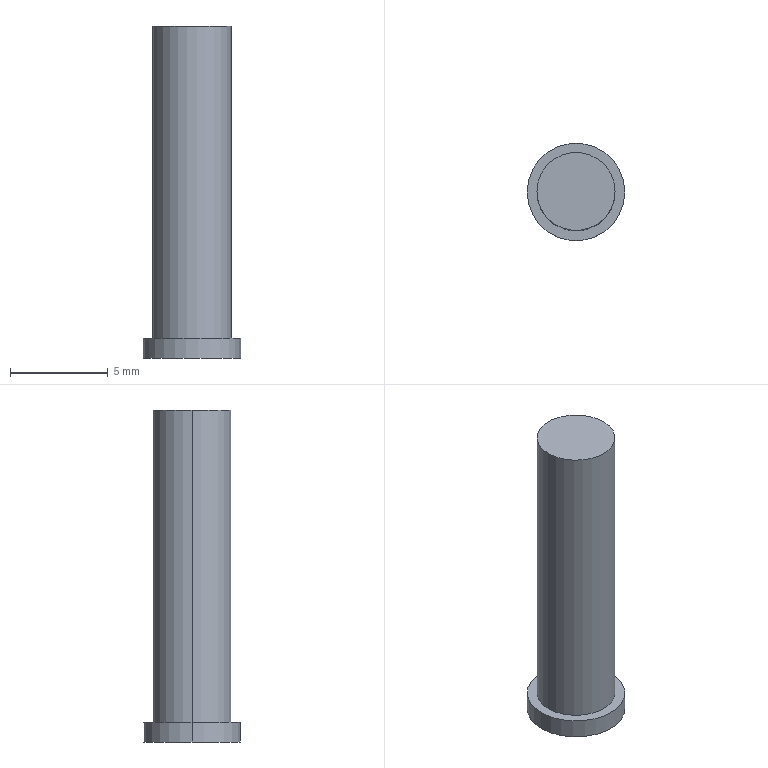Part | SolidWorks | features Extrusion 1, ICE 1 | 1 solid | 7 faces | box 5 x 5 x 17 mm | volume 220.697 mm3 | cylinder 4 | plane 3 | commonest cylinder face diameters 4 x2 5 x2
STEP:
#1=CARTESIAN_POINT('',(2.,0.,17.));
#2=VERTEX_POINT('',#1);
#3=CARTESIAN_POINT('',(-2.,0.,17.));
#4=VERTEX_POINT('',#3);
#5=CARTESIAN_POINT('',(0.,0.,17.));
#6=DIRECTION('',(0.,0.,1.));
#7=DIRECTION('',(1.,0.,0.));
#8=AXIS2_PLACEMENT_3D('',#5,#6,#7);
#9=CIRCLE('',#8,2.);
#10=EDGE_CURVE('',#2,#4,#9,.T.);
#11=ORIENTED_EDGE('',*,*,#10,.F.);
#12=CARTESIAN_POINT('',(2.,0.,1.));
#13=VERTEX_POINT('',#12);
#14=CARTESIAN_POINT('',(2.,0.,17.));
#15=DIRECTION('',(0.,0.,-1.));
#16=VECTOR('',#15,1000.);
#17=LINE('',#14,#16);
#18=EDGE_CURVE('',#2,#13,#17,.T.);
#19=ORIENTED_EDGE('',*,*,#18,.T.);
#20=CARTESIAN_POINT('',(-2.,0.,1.));
#21=VERTEX_POINT('',#20);
#22=CARTESIAN_POINT('',(0.,0.,1.));
#23=DIRECTION('',(0.,0.,1.));
#24=DIRECTION('',(1.,0.,0.));
#25=AXIS2_PLACEMENT_3D('',#22,#23,#24);
#26=CIRCLE('',#25,2.);
#27=EDGE_CURVE('',#13,#21,#26,.T.);
#28=ORIENTED_EDGE('',*,*,#27,.T.);
#29=CARTESIAN_POINT('',(-2.,0.,17.));
#30=DIRECTION('',(0.,0.,-1.));
#31=VECTOR('',#30,1000.);
#32=LINE('',#29,#31);
#33=EDGE_CURVE('',#4,#21,#32,.T.);
#34=ORIENTED_EDGE('',*,*,#33,.F.);
#35=EDGE_LOOP('',(#11,#19,#28,#34));
#36=FACE_OUTER_BOUND('',#35,.T.);
#37=CARTESIAN_POINT('',(0.,0.,17.));
#38=DIRECTION('',(0.,0.,-1.));
#39=DIRECTION('',(-1.,0.,0.));
#40=AXIS2_PLACEMENT_3D('',#37,#38,#39);
#41=CYLINDRICAL_SURFACE('',#40,2.);
#42=ADVANCED_FACE('',(#36),#41,.T.);
#43=CARTESIAN_POINT('',(2.5,0.,1.));
#44=VERTEX_POINT('',#43);
#45=CARTESIAN_POINT('',(-2.5,0.,1.));
#46=VERTEX_POINT('',#45);
#47=CARTESIAN_POINT('',(0.,0.,1.));
#48=DIRECTION('',(0.,0.,1.));
#49=DIRECTION('',(1.,0.,0.));
#50=AXIS2_PLACEMENT_3D('',#47,#48,#49);
#51=CIRCLE('',#50,2.5);
#52=EDGE_CURVE('',#44,#46,#51,.T.);
#53=ORIENTED_EDGE('',*,*,#52,.F.);
#54=CARTESIAN_POINT('',(2.5,0.,0.));
#55=VERTEX_POINT('',#54);
#56=CARTESIAN_POINT('',(2.5,0.,1.));
#57=DIRECTION('',(0.,0.,-1.));
#58=VECTOR('',#57,1000.);
#59=LINE('',#56,#58);
#60=EDGE_CURVE('',#44,#55,#59,.T.);
#61=ORIENTED_EDGE('',*,*,#60,.T.);
#62=CARTESIAN_POINT('',(-2.5,0.,0.));
#63=VERTEX_POINT('',#62);
#64=CARTESIAN_POINT('',(0.,0.,0.));
#65=DIRECTION('',(0.,0.,1.));
#66=DIRECTION('',(1.,0.,0.));
#67=AXIS2_PLACEMENT_3D('',#64,#65,#66);
#68=CIRCLE('',#67,2.5);
#69=EDGE_CURVE('',#55,#63,#68,.T.);
#70=ORIENTED_EDGE('',*,*,#69,.T.);
#71=CARTESIAN_POINT('',(-2.5,0.,1.));
#72=DIRECTION('',(0.,0.,-1.));
#73=VECTOR('',#72,1000.);
#74=LINE('',#71,#73);
#75=EDGE_CURVE('',#46,#63,#74,.T.);
#76=ORIENTED_EDGE('',*,*,#75,.F.);
#77=EDGE_LOOP('',(#53,#61,#70,#76));
#78=FACE_OUTER_BOUND('',#77,.T.);
#79=CARTESIAN_POINT('',(0.,0.,1.));
#80=DIRECTION('',(0.,0.,-1.));
#81=DIRECTION('',(-1.,0.,0.));
#82=AXIS2_PLACEMENT_3D('',#79,#80,#81);
#83=CYLINDRICAL_SURFACE('',#82,2.5);
#84=ADVANCED_FACE('',(#78),#83,.T.);
#85=ORIENTED_EDGE('',*,*,#60,.F.);
#86=CARTESIAN_POINT('',(0.,0.,1.));
#87=DIRECTION('',(0.,0.,1.));
#88=DIRECTION('',(1.,0.,0.));
#89=AXIS2_PLACEMENT_3D('',#86,#87,#88);
#90=CIRCLE('',#89,2.5);
#91=EDGE_CURVE('',#46,#44,#90,.T.);
#92=ORIENTED_EDGE('',*,*,#91,.F.);
#93=ORIENTED_EDGE('',*,*,#75,.T.);
#94=CARTESIAN_POINT('',(0.,0.,0.));
#95=DIRECTION('',(0.,0.,1.));
#96=DIRECTION('',(1.,0.,0.));
#97=AXIS2_PLACEMENT_3D('',#94,#95,#96);
#98=CIRCLE('',#97,2.5);
#99=EDGE_CURVE('',#63,#55,#98,.T.);
#100=ORIENTED_EDGE('',*,*,#99,.T.);
#101=EDGE_LOOP('',(#85,#92,#93,#100));
#102=FACE_OUTER_BOUND('',#101,.T.);
#103=CARTESIAN_POINT('',(0.,0.,1.));
#104=DIRECTION('',(0.,0.,-1.));
#105=DIRECTION('',(-1.,0.,0.));
#106=AXIS2_PLACEMENT_3D('',#103,#104,#105);
#107=CYLINDRICAL_SURFACE('',#106,2.5);
#108=ADVANCED_FACE('',(#102),#107,.T.);
#109=CARTESIAN_POINT('',(0.,0.,1.));
#110=DIRECTION('',(0.,0.,1.));
#111=DIRECTION('',(1.,0.,0.));
#112=AXIS2_PLACEMENT_3D('',#109,#110,#111);
#113=CIRCLE('',#112,2.);
#114=EDGE_CURVE('',#21,#13,#113,.T.);
#115=ORIENTED_EDGE('',*,*,#114,.F.);
#116=ORIENTED_EDGE('',*,*,#27,.F.);
#117=EDGE_LOOP('',(#115,#116));
#118=FACE_BOUND('',#117,.T.);
#119=ORIENTED_EDGE('',*,*,#91,.T.);
#120=ORIENTED_EDGE('',*,*,#52,.T.);
#121=EDGE_LOOP('',(#119,#120));
#122=FACE_OUTER_BOUND('',#121,.T.);
#123=CARTESIAN_POINT('',(0.,0.,1.));
#124=DIRECTION('',(0.,0.,1.));
#125=DIRECTION('',(1.,0.,0.));
#126=AXIS2_PLACEMENT_3D('',#123,#124,#125);
#127=PLANE('',#126);
#128=ADVANCED_FACE('',(#118,#122),#127,.T.);
#129=ORIENTED_EDGE('',*,*,#99,.F.);
#130=ORIENTED_EDGE('',*,*,#69,.F.);
#131=EDGE_LOOP('',(#129,#130));
#132=FACE_OUTER_BOUND('',#131,.T.);
#133=CARTESIAN_POINT('',(0.,0.,0.));
#134=DIRECTION('',(0.,0.,1.));
#135=DIRECTION('',(1.,0.,0.));
#136=AXIS2_PLACEMENT_3D('',#133,#134,#135);
#137=PLANE('',#136);
#138=ADVANCED_FACE('',(#132),#137,.F.);
#139=ORIENTED_EDGE('',*,*,#18,.F.);
#140=CARTESIAN_POINT('',(0.,0.,17.));
#141=DIRECTION('',(0.,0.,1.));
#142=DIRECTION('',(1.,0.,0.));
#143=AXIS2_PLACEMENT_3D('',#140,#141,#142);
#144=CIRCLE('',#143,2.);
#145=EDGE_CURVE('',#4,#2,#144,.T.);
#146=ORIENTED_EDGE('',*,*,#145,.F.);
#147=ORIENTED_EDGE('',*,*,#33,.T.);
#148=ORIENTED_EDGE('',*,*,#114,.T.);
#149=EDGE_LOOP('',(#139,#146,#147,#148));
#150=FACE_OUTER_BOUND('',#149,.T.);
#151=CARTESIAN_POINT('',(0.,0.,17.));
#152=DIRECTION('',(0.,0.,-1.));
#153=DIRECTION('',(-1.,0.,0.));
#154=AXIS2_PLACEMENT_3D('',#151,#152,#153);
#155=CYLINDRICAL_SURFACE('',#154,2.);
#156=ADVANCED_FACE('',(#150),#155,.T.);
#157=ORIENTED_EDGE('',*,*,#145,.T.);
#158=ORIENTED_EDGE('',*,*,#10,.T.);
#159=EDGE_LOOP('',(#157,#158));
#160=FACE_OUTER_BOUND('',#159,.T.);
#161=CARTESIAN_POINT('',(0.,0.,17.));
#162=DIRECTION('',(0.,0.,1.));
#163=DIRECTION('',(1.,0.,0.));
#164=AXIS2_PLACEMENT_3D('',#161,#162,#163);
#165=PLANE('',#164);
#166=ADVANCED_FACE('',(#160),#165,.T.);
#167=CLOSED_SHELL('',(#42,#84,#108,#128,#138,#156,#166));
#168=MANIFOLD_SOLID_BREP('',#167);
#169=CARTESIAN_POINT('',(0.,0.,0.));
#170=DIRECTION('',(0.,0.,1.));
#171=DIRECTION('',(1.,0.,0.));
#172=AXIS2_PLACEMENT_3D('',#169,#170,#171);
#173=(LENGTH_UNIT()NAMED_UNIT(*)SI_UNIT(.MILLI.,.METRE.));
#174=UNCERTAINTY_MEASURE_WITH_UNIT(LENGTH_MEASURE(0.00001),#173,'','');
#175=(NAMED_UNIT(*)PLANE_ANGLE_UNIT()SI_UNIT($,.RADIAN.));
#176=(NAMED_UNIT(*)SI_UNIT($,.STERADIAN.)SOLID_ANGLE_UNIT());
#177=(GEOMETRIC_REPRESENTATION_CONTEXT(3)GLOBAL_UNCERTAINTY_ASSIGNED_CONTEXT((#174))GLOBAL_UNIT_ASSIGNED_CONTEXT((#173,#175,#176))REPRESENTATION_CONTEXT('',''));
#178=ADVANCED_BREP_SHAPE_REPRESENTATION('',(#168,#172),#177);